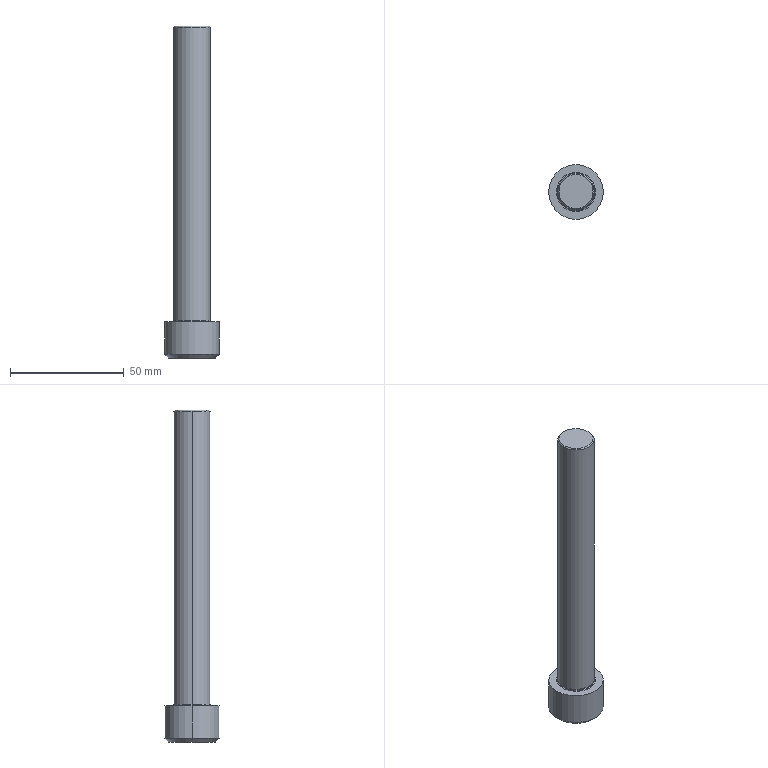Part | Creo | 1 solid | 23 faces | box 24 x 24 x 146 mm | volume 31613 mm3 | plane 9 | cone 6 | cylinder 4 | torus 4 | commonest cylinder face diameters 16 x2 24 x2
STEP:
#1=CARTESIAN_POINT('',(0.,0.,0.));
#2=DIRECTION('',(0.,0.,1.));
#3=DIRECTION('',(1.,0.,0.));
#4=AXIS2_PLACEMENT_3D('',#1,#2,#3);
#5=CARTESIAN_POINT('',(101.917,220.,10.5));
#6=VERTEX_POINT('',#5);
#7=CARTESIAN_POINT('',(105.959,227.,10.5));
#8=VERTEX_POINT('',#7);
#9=CARTESIAN_POINT('',(101.917,220.,10.5));
#10=CARTESIAN_POINT('',(102.137,220.381,10.627));
#11=CARTESIAN_POINT('',(102.578,221.145,10.851));
#12=CARTESIAN_POINT('',(103.254,222.315,11.073));
#13=CARTESIAN_POINT('',(103.936,223.496,11.151));
#14=CARTESIAN_POINT('',(104.621,224.683,11.073));
#15=CARTESIAN_POINT('',(105.295,225.85,10.852));
#16=CARTESIAN_POINT('',(105.738,226.618,10.627));
#17=CARTESIAN_POINT('',(105.959,227.,10.5));
#18=B_SPLINE_CURVE_WITH_KNOTS('',3,(#9,#10,#11,#12,#13,#14,#15,#16,#17),.UNSPECIFIED.,.F.,.F.,(4,1,1,1,1,1,4),(0.,0.1667,0.3333,0.5,0.6667,0.8333,1.),.UNSPECIFIED.);
#19=EDGE_CURVE('',#6,#8,#18,.T.);
#20=ORIENTED_EDGE('',*,*,#19,.F.);
#21=CARTESIAN_POINT('',(110.,220.,15.167));
#22=VERTEX_POINT('',#21);
#23=CARTESIAN_POINT('',(110.,220.,15.167));
#24=DIRECTION('',(-0.866,0.,-0.5));
#25=VECTOR('',#24,9.333);
#26=LINE('',#23,#25);
#27=EDGE_CURVE('',#22,#6,#26,.T.);
#28=ORIENTED_EDGE('',*,*,#27,.F.);
#29=CARTESIAN_POINT('',(118.083,220.,10.5));
#30=VERTEX_POINT('',#29);
#31=CARTESIAN_POINT('',(110.,220.,15.167));
#32=DIRECTION('',(0.866,0.,-0.5));
#33=VECTOR('',#32,9.333);
#34=LINE('',#31,#33);
#35=EDGE_CURVE('',#22,#30,#34,.T.);
#36=ORIENTED_EDGE('',*,*,#35,.T.);
#37=CARTESIAN_POINT('',(114.041,227.,10.5));
#38=VERTEX_POINT('',#37);
#39=CARTESIAN_POINT('',(114.041,227.,10.5));
#40=CARTESIAN_POINT('',(114.261,226.619,10.627));
#41=CARTESIAN_POINT('',(114.703,225.855,10.851));
#42=CARTESIAN_POINT('',(115.378,224.685,11.073));
#43=CARTESIAN_POINT('',(116.06,223.504,11.151));
#44=CARTESIAN_POINT('',(116.745,222.317,11.073));
#45=CARTESIAN_POINT('',(117.419,221.15,10.852));
#46=CARTESIAN_POINT('',(117.862,220.382,10.627));
#47=CARTESIAN_POINT('',(118.083,220.,10.5));
#48=B_SPLINE_CURVE_WITH_KNOTS('',3,(#39,#40,#41,#42,#43,#44,#45,#46,#47),.UNSPECIFIED.,.F.,.F.,(4,1,1,1,1,1,4),(0.,0.1667,0.3333,0.5,0.6667,0.8333,1.),.UNSPECIFIED.);
#49=EDGE_CURVE('',#38,#30,#48,.T.);
#50=ORIENTED_EDGE('',*,*,#49,.F.);
#51=CARTESIAN_POINT('',(105.959,227.,10.5));
#52=CARTESIAN_POINT('',(106.396,227.,10.626));
#53=CARTESIAN_POINT('',(107.277,227.,10.85));
#54=CARTESIAN_POINT('',(108.631,227.,11.073));
#55=CARTESIAN_POINT('',(109.998,227.,11.151));
#56=CARTESIAN_POINT('',(111.363,227.,11.074));
#57=CARTESIAN_POINT('',(112.717,227.,10.851));
#58=CARTESIAN_POINT('',(113.601,227.,10.627));
#59=CARTESIAN_POINT('',(114.041,227.,10.5));
#60=B_SPLINE_CURVE_WITH_KNOTS('',3,(#51,#52,#53,#54,#55,#56,#57,#58,#59),.UNSPECIFIED.,.F.,.F.,(4,1,1,1,1,1,4),(0.,0.1667,0.3333,0.5,0.6667,0.8333,1.),.UNSPECIFIED.);
#61=EDGE_CURVE('',#8,#38,#60,.T.);
#62=ORIENTED_EDGE('',*,*,#61,.F.);
#63=EDGE_LOOP('',(#20,#28,#36,#50,#62));
#64=FACE_OUTER_BOUND('',#63,.F.);
#65=CARTESIAN_POINT('',(110.,220.,12.787));
#66=DIRECTION('',(0.,0.,-1.));
#67=DIRECTION('',(-1.,0.,0.));
#68=AXIS2_PLACEMENT_3D('',#65,#66,#67);
#69=CONICAL_SURFACE('',#68,4.122,60.);
#70=ADVANCED_FACE('',(#64),#69,.F.);
#71=CARTESIAN_POINT('',(105.959,227.,2.5));
#72=VERTEX_POINT('',#71);
#73=CARTESIAN_POINT('',(101.917,220.,2.5));
#74=VERTEX_POINT('',#73);
#75=CARTESIAN_POINT('',(105.959,227.,2.5));
#76=DIRECTION('',(-0.5,-0.866,0.));
#77=VECTOR('',#76,8.083);
#78=LINE('',#75,#77);
#79=EDGE_CURVE('',#72,#74,#78,.T.);
#80=ORIENTED_EDGE('',*,*,#79,.T.);
#81=CARTESIAN_POINT('',(101.917,220.,2.5));
#82=DIRECTION('',(0.,0.,1.));
#83=VECTOR('',#82,8.);
#84=LINE('',#81,#83);
#85=EDGE_CURVE('',#74,#6,#84,.T.);
#86=ORIENTED_EDGE('',*,*,#85,.T.);
#87=ORIENTED_EDGE('',*,*,#19,.T.);
#88=CARTESIAN_POINT('',(105.959,227.,2.5));
#89=DIRECTION('',(0.,0.,1.));
#90=VECTOR('',#89,8.);
#91=LINE('',#88,#90);
#92=EDGE_CURVE('',#72,#8,#91,.T.);
#93=ORIENTED_EDGE('',*,*,#92,.F.);
#94=EDGE_LOOP('',(#80,#86,#87,#93));
#95=FACE_OUTER_BOUND('',#94,.F.);
#96=CARTESIAN_POINT('',(105.959,227.,10.5));
#97=DIRECTION('',(0.866,-0.5,0.));
#98=DIRECTION('',(-0.5,-0.866,0.));
#99=AXIS2_PLACEMENT_3D('',#96,#97,#98);
#100=PLANE('',#99);
#101=ADVANCED_FACE('',(#95),#100,.T.);
#102=CARTESIAN_POINT('',(99.6,220.,2.5));
#103=VERTEX_POINT('',#102);
#104=CARTESIAN_POINT('',(120.4,220.,2.5));
#105=VERTEX_POINT('',#104);
#106=CARTESIAN_POINT('',(110.,220.,2.5));
#107=DIRECTION('',(0.,0.,-1.));
#108=DIRECTION('',(-1.,0.,0.));
#109=AXIS2_PLACEMENT_3D('',#106,#107,#108);
#110=CIRCLE('',#109,10.4);
#111=EDGE_CURVE('',#103,#105,#110,.T.);
#112=ORIENTED_EDGE('',*,*,#111,.F.);
#113=CARTESIAN_POINT('',(110.,220.,2.5));
#114=DIRECTION('',(0.,0.,-1.));
#115=DIRECTION('',(1.,0.,0.));
#116=AXIS2_PLACEMENT_3D('',#113,#114,#115);
#117=CIRCLE('',#116,10.4);
#118=EDGE_CURVE('',#105,#103,#117,.T.);
#119=ORIENTED_EDGE('',*,*,#118,.F.);
#120=EDGE_LOOP('',(#112,#119));
#121=FACE_OUTER_BOUND('',#120,.F.);
#122=CARTESIAN_POINT('',(105.959,213.,2.5));
#123=VERTEX_POINT('',#122);
#124=CARTESIAN_POINT('',(101.917,220.,2.5));
#125=DIRECTION('',(0.5,-0.866,0.));
#126=VECTOR('',#125,8.083);
#127=LINE('',#124,#126);
#128=EDGE_CURVE('',#74,#123,#127,.T.);
#129=ORIENTED_EDGE('',*,*,#128,.F.);
#130=ORIENTED_EDGE('',*,*,#79,.F.);
#131=CARTESIAN_POINT('',(114.041,227.,2.5));
#132=VERTEX_POINT('',#131);
#133=CARTESIAN_POINT('',(105.959,227.,2.5));
#134=DIRECTION('',(1.,0.,0.));
#135=VECTOR('',#134,8.083);
#136=LINE('',#133,#135);
#137=EDGE_CURVE('',#72,#132,#136,.T.);
#138=ORIENTED_EDGE('',*,*,#137,.T.);
#139=CARTESIAN_POINT('',(118.083,220.,2.5));
#140=VERTEX_POINT('',#139);
#141=CARTESIAN_POINT('',(118.083,220.,2.5));
#142=DIRECTION('',(-0.5,0.866,0.));
#143=VECTOR('',#142,8.083);
#144=LINE('',#141,#143);
#145=EDGE_CURVE('',#140,#132,#144,.T.);
#146=ORIENTED_EDGE('',*,*,#145,.F.);
#147=CARTESIAN_POINT('',(114.041,213.,2.5));
#148=VERTEX_POINT('',#147);
#149=CARTESIAN_POINT('',(114.041,213.,2.5));
#150=DIRECTION('',(0.5,0.866,0.));
#151=VECTOR('',#150,8.083);
#152=LINE('',#149,#151);
#153=EDGE_CURVE('',#148,#140,#152,.T.);
#154=ORIENTED_EDGE('',*,*,#153,.F.);
#155=CARTESIAN_POINT('',(114.041,213.,2.5));
#156=DIRECTION('',(-1.,0.,0.));
#157=VECTOR('',#156,8.083);
#158=LINE('',#155,#157);
#159=EDGE_CURVE('',#148,#123,#158,.T.);
#160=ORIENTED_EDGE('',*,*,#159,.T.);
#161=EDGE_LOOP('',(#129,#130,#138,#146,#154,#160));
#162=FACE_BOUND('',#161,.F.);
#163=CARTESIAN_POINT('',(110.,220.,2.5));
#164=DIRECTION('',(0.,0.,-1.));
#165=DIRECTION('',(-1.,0.,0.));
#166=AXIS2_PLACEMENT_3D('',#163,#164,#165);
#167=PLANE('',#166);
#168=ADVANCED_FACE('',(#121,#162),#167,.T.);
#169=CARTESIAN_POINT('',(98.,220.,4.1));
#170=VERTEX_POINT('',#169);
#171=CARTESIAN_POINT('',(122.,220.,4.1));
#172=VERTEX_POINT('',#171);
#173=CARTESIAN_POINT('',(110.,220.,4.1));
#174=DIRECTION('',(0.,0.,-1.));
#175=DIRECTION('',(-1.,0.,0.));
#176=AXIS2_PLACEMENT_3D('',#173,#174,#175);
#177=CIRCLE('',#176,12.);
#178=EDGE_CURVE('',#170,#172,#177,.T.);
#179=ORIENTED_EDGE('',*,*,#178,.F.);
#180=CARTESIAN_POINT('',(99.6,220.,2.5));
#181=DIRECTION('',(-0.7071,0.,0.7071));
#182=VECTOR('',#181,2.263);
#183=LINE('',#180,#182);
#184=EDGE_CURVE('',#103,#170,#183,.T.);
#185=ORIENTED_EDGE('',*,*,#184,.F.);
#186=ORIENTED_EDGE('',*,*,#111,.T.);
#187=CARTESIAN_POINT('',(120.4,220.,2.5));
#188=DIRECTION('',(0.7071,0.,0.7071));
#189=VECTOR('',#188,2.263);
#190=LINE('',#187,#189);
#191=EDGE_CURVE('',#105,#172,#190,.T.);
#192=ORIENTED_EDGE('',*,*,#191,.T.);
#193=EDGE_LOOP('',(#179,#185,#186,#192));
#194=FACE_OUTER_BOUND('',#193,.F.);
#195=CARTESIAN_POINT('',(110.,220.,3.3));
#196=DIRECTION('',(0.,0.,1.));
#197=DIRECTION('',(1.,0.,0.));
#198=AXIS2_PLACEMENT_3D('',#195,#196,#197);
#199=CONICAL_SURFACE('',#198,11.2,45.);
#200=ADVANCED_FACE('',(#194),#199,.T.);
#201=ORIENTED_EDGE('',*,*,#178,.T.);
#202=CARTESIAN_POINT('',(122.,220.,18.5));
#203=VERTEX_POINT('',#202);
#204=CARTESIAN_POINT('',(122.,220.,18.5));
#205=DIRECTION('',(0.,0.,-1.));
#206=VECTOR('',#205,14.4);
#207=LINE('',#204,#206);
#208=EDGE_CURVE('',#203,#172,#207,.T.);
#209=ORIENTED_EDGE('',*,*,#208,.F.);
#210=CARTESIAN_POINT('',(98.,220.,18.5));
#211=VERTEX_POINT('',#210);
#212=CARTESIAN_POINT('',(110.,220.,18.5));
#213=DIRECTION('',(0.,0.,1.));
#214=DIRECTION('',(1.,0.,0.));
#215=AXIS2_PLACEMENT_3D('',#212,#213,#214);
#216=CIRCLE('',#215,12.);
#217=EDGE_CURVE('',#203,#211,#216,.T.);
#218=ORIENTED_EDGE('',*,*,#217,.T.);
#219=CARTESIAN_POINT('',(98.,220.,18.5));
#220=DIRECTION('',(0.,0.,-1.));
#221=VECTOR('',#220,14.4);
#222=LINE('',#219,#221);
#223=EDGE_CURVE('',#211,#170,#222,.T.);
#224=ORIENTED_EDGE('',*,*,#223,.T.);
#225=EDGE_LOOP('',(#201,#209,#218,#224));
#226=FACE_OUTER_BOUND('',#225,.F.);
#227=CARTESIAN_POINT('',(110.,220.,18.5));
#228=DIRECTION('',(0.,0.,-1.));
#229=DIRECTION('',(-1.,0.,0.));
#230=AXIS2_PLACEMENT_3D('',#227,#228,#229);
#231=CYLINDRICAL_SURFACE('',#230,12.);
#232=ADVANCED_FACE('',(#226),#231,.T.);
#233=CARTESIAN_POINT('',(110.,220.,4.1));
#234=DIRECTION('',(0.,0.,-1.));
#235=DIRECTION('',(1.,0.,0.));
#236=AXIS2_PLACEMENT_3D('',#233,#234,#235);
#237=CIRCLE('',#236,12.);
#238=EDGE_CURVE('',#172,#170,#237,.T.);
#239=ORIENTED_EDGE('',*,*,#238,.T.);
#240=ORIENTED_EDGE('',*,*,#223,.F.);
#241=CARTESIAN_POINT('',(110.,220.,18.5));
#242=DIRECTION('',(0.,0.,1.));
#243=DIRECTION('',(-1.,0.,0.));
#244=AXIS2_PLACEMENT_3D('',#241,#242,#243);
#245=CIRCLE('',#244,12.);
#246=EDGE_CURVE('',#211,#203,#245,.T.);
#247=ORIENTED_EDGE('',*,*,#246,.T.);
#248=ORIENTED_EDGE('',*,*,#208,.T.);
#249=EDGE_LOOP('',(#239,#240,#247,#248));
#250=FACE_OUTER_BOUND('',#249,.F.);
#251=CARTESIAN_POINT('',(110.,220.,18.5));
#252=DIRECTION('',(0.,0.,-1.));
#253=DIRECTION('',(-1.,0.,0.));
#254=AXIS2_PLACEMENT_3D('',#251,#252,#253);
#255=CYLINDRICAL_SURFACE('',#254,12.);
#256=ADVANCED_FACE('',(#250),#255,.T.);
#257=ORIENTED_EDGE('',*,*,#238,.F.);
#258=ORIENTED_EDGE('',*,*,#191,.F.);
#259=ORIENTED_EDGE('',*,*,#118,.T.);
#260=ORIENTED_EDGE('',*,*,#184,.T.);
#261=EDGE_LOOP('',(#257,#258,#259,#260));
#262=FACE_OUTER_BOUND('',#261,.F.);
#263=CARTESIAN_POINT('',(110.,220.,3.3));
#264=DIRECTION('',(0.,0.,1.));
#265=DIRECTION('',(1.,0.,0.));
#266=AXIS2_PLACEMENT_3D('',#263,#264,#265);
#267=CONICAL_SURFACE('',#266,11.2,45.);
#268=ADVANCED_FACE('',(#262),#267,.T.);
#269=ORIENTED_EDGE('',*,*,#246,.F.);
#270=ORIENTED_EDGE('',*,*,#217,.F.);
#271=EDGE_LOOP('',(#269,#270));
#272=FACE_OUTER_BOUND('',#271,.F.);
#273=CARTESIAN_POINT('',(101.4,220.,18.5));
#274=VERTEX_POINT('',#273);
#275=CARTESIAN_POINT('',(118.6,220.,18.5));
#276=VERTEX_POINT('',#275);
#277=CARTESIAN_POINT('',(110.,220.,18.5));
#278=DIRECTION('',(0.,0.,-1.));
#279=DIRECTION('',(-1.,0.,0.));
#280=AXIS2_PLACEMENT_3D('',#277,#278,#279);
#281=CIRCLE('',#280,8.6);
#282=EDGE_CURVE('',#274,#276,#281,.T.);
#283=ORIENTED_EDGE('',*,*,#282,.F.);
#284=CARTESIAN_POINT('',(110.,220.,18.5));
#285=DIRECTION('',(0.,0.,-1.));
#286=DIRECTION('',(1.,0.,0.));
#287=AXIS2_PLACEMENT_3D('',#284,#285,#286);
#288=CIRCLE('',#287,8.6);
#289=EDGE_CURVE('',#276,#274,#288,.T.);
#290=ORIENTED_EDGE('',*,*,#289,.F.);
#291=EDGE_LOOP('',(#283,#290));
#292=FACE_BOUND('',#291,.F.);
#293=CARTESIAN_POINT('',(110.,220.,18.5));
#294=DIRECTION('',(0.,0.,-1.));
#295=DIRECTION('',(-1.,0.,0.));
#296=AXIS2_PLACEMENT_3D('',#293,#294,#295);
#297=PLANE('',#296);
#298=ADVANCED_FACE('',(#272,#292),#297,.F.);
#299=ORIENTED_EDGE('',*,*,#282,.T.);
#300=CARTESIAN_POINT('',(118.176,220.,18.676));
#301=VERTEX_POINT('',#300);
#302=CARTESIAN_POINT('',(118.6,220.,19.1));
#303=DIRECTION('',(0.,1.,0.));
#304=DIRECTION('',(0.,0.,-1.));
#305=AXIS2_PLACEMENT_3D('',#302,#303,#304);
#306=CIRCLE('',#305,0.6);
#307=EDGE_CURVE('',#276,#301,#306,.T.);
#308=ORIENTED_EDGE('',*,*,#307,.T.);
#309=CARTESIAN_POINT('',(101.824,220.,18.676));
#310=VERTEX_POINT('',#309);
#311=CARTESIAN_POINT('',(110.,220.,18.676));
#312=DIRECTION('',(0.,0.,-1.));
#313=DIRECTION('',(-1.,0.,0.));
#314=AXIS2_PLACEMENT_3D('',#311,#312,#313);
#315=CIRCLE('',#314,8.176);
#316=EDGE_CURVE('',#310,#301,#315,.T.);
#317=ORIENTED_EDGE('',*,*,#316,.F.);
#318=CARTESIAN_POINT('',(101.4,220.,19.1));
#319=DIRECTION('',(0.,-1.,0.));
#320=DIRECTION('',(0.,0.,-1.));
#321=AXIS2_PLACEMENT_3D('',#318,#319,#320);
#322=CIRCLE('',#321,0.6);
#323=EDGE_CURVE('',#274,#310,#322,.T.);
#324=ORIENTED_EDGE('',*,*,#323,.F.);
#325=EDGE_LOOP('',(#299,#308,#317,#324));
#326=FACE_OUTER_BOUND('',#325,.F.);
#327=CARTESIAN_POINT('',(110.,220.,19.1));
#328=DIRECTION('',(0.,0.,-1.));
#329=DIRECTION('',(-1.,0.,0.));
#330=AXIS2_PLACEMENT_3D('',#327,#328,#329);
#331=TOROIDAL_SURFACE('',#330,8.6,0.6);
#332=ADVANCED_FACE('',(#326),#331,.F.);
#333=ORIENTED_EDGE('',*,*,#289,.T.);
#334=ORIENTED_EDGE('',*,*,#323,.T.);
#335=CARTESIAN_POINT('',(110.,220.,18.676));
#336=DIRECTION('',(0.,0.,-1.));
#337=DIRECTION('',(1.,0.,0.));
#338=AXIS2_PLACEMENT_3D('',#335,#336,#337);
#339=CIRCLE('',#338,8.176);
#340=EDGE_CURVE('',#301,#310,#339,.T.);
#341=ORIENTED_EDGE('',*,*,#340,.F.);
#342=ORIENTED_EDGE('',*,*,#307,.F.);
#343=EDGE_LOOP('',(#333,#334,#341,#342));
#344=FACE_OUTER_BOUND('',#343,.F.);
#345=CARTESIAN_POINT('',(110.,220.,19.1));
#346=DIRECTION('',(0.,0.,-1.));
#347=DIRECTION('',(-1.,0.,0.));
#348=AXIS2_PLACEMENT_3D('',#345,#346,#347);
#349=TOROIDAL_SURFACE('',#348,8.6,0.6);
#350=ADVANCED_FACE('',(#344),#349,.F.);
#351=CARTESIAN_POINT('',(118.,220.,19.1));
#352=VERTEX_POINT('',#351);
#353=CARTESIAN_POINT('',(102.,220.,19.1));
#354=VERTEX_POINT('',#353);
#355=CARTESIAN_POINT('',(110.,220.,19.1));
#356=DIRECTION('',(0.,0.,-1.));
#357=DIRECTION('',(1.,0.,0.));
#358=AXIS2_PLACEMENT_3D('',#355,#356,#357);
#359=CIRCLE('',#358,8.);
#360=EDGE_CURVE('',#352,#354,#359,.T.);
#361=ORIENTED_EDGE('',*,*,#360,.F.);
#362=CARTESIAN_POINT('',(118.6,220.,19.1));
#363=DIRECTION('',(0.,1.,0.));
#364=DIRECTION('',(-0.7071,0.,-0.7071));
#365=AXIS2_PLACEMENT_3D('',#362,#363,#364);
#366=CIRCLE('',#365,0.6);
#367=EDGE_CURVE('',#301,#352,#366,.T.);
#368=ORIENTED_EDGE('',*,*,#367,.F.);
#369=ORIENTED_EDGE('',*,*,#340,.T.);
#370=CARTESIAN_POINT('',(101.4,220.,19.1));
#371=DIRECTION('',(0.,-1.,0.));
#372=DIRECTION('',(0.7071,0.,-0.7071));
#373=AXIS2_PLACEMENT_3D('',#370,#371,#372);
#374=CIRCLE('',#373,0.6);
#375=EDGE_CURVE('',#310,#354,#374,.T.);
#376=ORIENTED_EDGE('',*,*,#375,.T.);
#377=EDGE_LOOP('',(#361,#368,#369,#376));
#378=FACE_OUTER_BOUND('',#377,.F.);
#379=CARTESIAN_POINT('',(110.,220.,19.1));
#380=DIRECTION('',(0.,0.,-1.));
#381=DIRECTION('',(-1.,0.,0.));
#382=AXIS2_PLACEMENT_3D('',#379,#380,#381);
#383=TOROIDAL_SURFACE('',#382,8.6,0.6);
#384=ADVANCED_FACE('',(#378),#383,.F.);
#385=CARTESIAN_POINT('',(102.,220.,148.));
#386=VERTEX_POINT('',#385);
#387=CARTESIAN_POINT('',(118.,220.,148.));
#388=VERTEX_POINT('',#387);
#389=CARTESIAN_POINT('',(110.,220.,148.));
#390=DIRECTION('',(0.,0.,1.));
#391=DIRECTION('',(-1.,0.,0.));
#392=AXIS2_PLACEMENT_3D('',#389,#390,#391);
#393=CIRCLE('',#392,8.);
#394=EDGE_CURVE('',#386,#388,#393,.T.);
#395=ORIENTED_EDGE('',*,*,#394,.T.);
#396=CARTESIAN_POINT('',(118.,220.,148.));
#397=DIRECTION('',(0.,0.,-1.));
#398=VECTOR('',#397,128.9);
#399=LINE('',#396,#398);
#400=EDGE_CURVE('',#388,#352,#399,.T.);
#401=ORIENTED_EDGE('',*,*,#400,.T.);
#402=ORIENTED_EDGE('',*,*,#360,.T.);
#403=CARTESIAN_POINT('',(102.,220.,148.));
#404=DIRECTION('',(0.,0.,-1.));
#405=VECTOR('',#404,128.9);
#406=LINE('',#403,#405);
#407=EDGE_CURVE('',#386,#354,#406,.T.);
#408=ORIENTED_EDGE('',*,*,#407,.F.);
#409=EDGE_LOOP('',(#395,#401,#402,#408));
#410=FACE_OUTER_BOUND('',#409,.F.);
#411=CARTESIAN_POINT('',(110.,220.,148.5));
#412=DIRECTION('',(0.,0.,-1.));
#413=DIRECTION('',(-1.,0.,0.));
#414=AXIS2_PLACEMENT_3D('',#411,#412,#413);
#415=CYLINDRICAL_SURFACE('',#414,8.);
#416=ADVANCED_FACE('',(#410),#415,.T.);
#417=CARTESIAN_POINT('',(102.5,220.,148.5));
#418=VERTEX_POINT('',#417);
#419=CARTESIAN_POINT('',(117.5,220.,148.5));
#420=VERTEX_POINT('',#419);
#421=CARTESIAN_POINT('',(110.,220.,148.5));
#422=DIRECTION('',(0.,0.,1.));
#423=DIRECTION('',(-1.,0.,0.));
#424=AXIS2_PLACEMENT_3D('',#421,#422,#423);
#425=CIRCLE('',#424,7.5);
#426=EDGE_CURVE('',#418,#420,#425,.T.);
#427=ORIENTED_EDGE('',*,*,#426,.T.);
#428=CARTESIAN_POINT('',(117.5,220.,148.5));
#429=DIRECTION('',(0.7071,0.,-0.7071));
#430=VECTOR('',#429,0.7071);
#431=LINE('',#428,#430);
#432=EDGE_CURVE('',#420,#388,#431,.T.);
#433=ORIENTED_EDGE('',*,*,#432,.T.);
#434=ORIENTED_EDGE('',*,*,#394,.F.);
#435=CARTESIAN_POINT('',(102.5,220.,148.5));
#436=DIRECTION('',(-0.7071,0.,-0.7071));
#437=VECTOR('',#436,0.7071);
#438=LINE('',#435,#437);
#439=EDGE_CURVE('',#418,#386,#438,.T.);
#440=ORIENTED_EDGE('',*,*,#439,.F.);
#441=EDGE_LOOP('',(#427,#433,#434,#440));
#442=FACE_OUTER_BOUND('',#441,.F.);
#443=CARTESIAN_POINT('',(110.,220.,148.25));
#444=DIRECTION('',(0.,0.,-1.));
#445=DIRECTION('',(-1.,0.,0.));
#446=AXIS2_PLACEMENT_3D('',#443,#444,#445);
#447=CONICAL_SURFACE('',#446,7.75,45.);
#448=ADVANCED_FACE('',(#442),#447,.T.);
#449=ORIENTED_EDGE('',*,*,#426,.F.);
#450=CARTESIAN_POINT('',(110.,220.,148.5));
#451=DIRECTION('',(0.,0.,1.));
#452=DIRECTION('',(1.,0.,0.));
#453=AXIS2_PLACEMENT_3D('',#450,#451,#452);
#454=CIRCLE('',#453,7.5);
#455=EDGE_CURVE('',#420,#418,#454,.T.);
#456=ORIENTED_EDGE('',*,*,#455,.F.);
#457=EDGE_LOOP('',(#449,#456));
#458=FACE_OUTER_BOUND('',#457,.F.);
#459=CARTESIAN_POINT('',(110.,220.,148.5));
#460=DIRECTION('',(0.,0.,-1.));
#461=DIRECTION('',(-1.,0.,0.));
#462=AXIS2_PLACEMENT_3D('',#459,#460,#461);
#463=PLANE('',#462);
#464=ADVANCED_FACE('',(#458),#463,.F.);
#465=ORIENTED_EDGE('',*,*,#455,.T.);
#466=ORIENTED_EDGE('',*,*,#439,.T.);
#467=CARTESIAN_POINT('',(110.,220.,148.));
#468=DIRECTION('',(0.,0.,1.));
#469=DIRECTION('',(1.,0.,0.));
#470=AXIS2_PLACEMENT_3D('',#467,#468,#469);
#471=CIRCLE('',#470,8.);
#472=EDGE_CURVE('',#388,#386,#471,.T.);
#473=ORIENTED_EDGE('',*,*,#472,.F.);
#474=ORIENTED_EDGE('',*,*,#432,.F.);
#475=EDGE_LOOP('',(#465,#466,#473,#474));
#476=FACE_OUTER_BOUND('',#475,.F.);
#477=CARTESIAN_POINT('',(110.,220.,148.25));
#478=DIRECTION('',(0.,0.,-1.));
#479=DIRECTION('',(-1.,0.,0.));
#480=AXIS2_PLACEMENT_3D('',#477,#478,#479);
#481=CONICAL_SURFACE('',#480,7.75,45.);
#482=ADVANCED_FACE('',(#476),#481,.T.);
#483=ORIENTED_EDGE('',*,*,#472,.T.);
#484=ORIENTED_EDGE('',*,*,#407,.T.);
#485=CARTESIAN_POINT('',(110.,220.,19.1));
#486=DIRECTION('',(0.,0.,-1.));
#487=DIRECTION('',(-1.,0.,0.));
#488=AXIS2_PLACEMENT_3D('',#485,#486,#487);
#489=CIRCLE('',#488,8.);
#490=EDGE_CURVE('',#354,#352,#489,.T.);
#491=ORIENTED_EDGE('',*,*,#490,.T.);
#492=ORIENTED_EDGE('',*,*,#400,.F.);
#493=EDGE_LOOP('',(#483,#484,#491,#492));
#494=FACE_OUTER_BOUND('',#493,.F.);
#495=CARTESIAN_POINT('',(110.,220.,148.5));
#496=DIRECTION('',(0.,0.,-1.));
#497=DIRECTION('',(-1.,0.,0.));
#498=AXIS2_PLACEMENT_3D('',#495,#496,#497);
#499=CYLINDRICAL_SURFACE('',#498,8.);
#500=ADVANCED_FACE('',(#494),#499,.T.);
#501=ORIENTED_EDGE('',*,*,#490,.F.);
#502=ORIENTED_EDGE('',*,*,#375,.F.);
#503=ORIENTED_EDGE('',*,*,#316,.T.);
#504=ORIENTED_EDGE('',*,*,#367,.T.);
#505=EDGE_LOOP('',(#501,#502,#503,#504));
#506=FACE_OUTER_BOUND('',#505,.F.);
#507=CARTESIAN_POINT('',(110.,220.,19.1));
#508=DIRECTION('',(0.,0.,-1.));
#509=DIRECTION('',(-1.,0.,0.));
#510=AXIS2_PLACEMENT_3D('',#507,#508,#509);
#511=TOROIDAL_SURFACE('',#510,8.6,0.6);
#512=ADVANCED_FACE('',(#506),#511,.F.);
#513=ORIENTED_EDGE('',*,*,#128,.T.);
#514=CARTESIAN_POINT('',(105.959,213.,10.5));
#515=VERTEX_POINT('',#514);
#516=CARTESIAN_POINT('',(105.959,213.,2.5));
#517=DIRECTION('',(0.,0.,1.));
#518=VECTOR('',#517,8.);
#519=LINE('',#516,#518);
#520=EDGE_CURVE('',#123,#515,#519,.T.);
#521=ORIENTED_EDGE('',*,*,#520,.T.);
#522=CARTESIAN_POINT('',(105.959,213.,10.5));
#523=CARTESIAN_POINT('',(105.739,213.381,10.627));
#524=CARTESIAN_POINT('',(105.297,214.145,10.851));
#525=CARTESIAN_POINT('',(104.622,215.315,11.073));
#526=CARTESIAN_POINT('',(103.94,216.496,11.151));
#527=CARTESIAN_POINT('',(103.255,217.683,11.073));
#528=CARTESIAN_POINT('',(102.581,218.85,10.852));
#529=CARTESIAN_POINT('',(102.138,219.618,10.627));
#530=CARTESIAN_POINT('',(101.917,220.,10.5));
#531=B_SPLINE_CURVE_WITH_KNOTS('',3,(#522,#523,#524,#525,#526,#527,#528,#529,#530),.UNSPECIFIED.,.F.,.F.,(4,1,1,1,1,1,4),(0.,0.1667,0.3333,0.5,0.6667,0.8333,1.),.UNSPECIFIED.);
#532=EDGE_CURVE('',#515,#6,#531,.T.);
#533=ORIENTED_EDGE('',*,*,#532,.T.);
#534=ORIENTED_EDGE('',*,*,#85,.F.);
#535=EDGE_LOOP('',(#513,#521,#533,#534));
#536=FACE_OUTER_BOUND('',#535,.F.);
#537=CARTESIAN_POINT('',(101.917,220.,10.5));
#538=DIRECTION('',(0.866,0.5,0.));
#539=DIRECTION('',(0.5,-0.866,0.));
#540=AXIS2_PLACEMENT_3D('',#537,#538,#539);
#541=PLANE('',#540);
#542=ADVANCED_FACE('',(#536),#541,.T.);
#543=ORIENTED_EDGE('',*,*,#159,.F.);
#544=CARTESIAN_POINT('',(114.041,213.,10.5));
#545=VERTEX_POINT('',#544);
#546=CARTESIAN_POINT('',(114.041,213.,2.5));
#547=DIRECTION('',(0.,0.,1.));
#548=VECTOR('',#547,8.);
#549=LINE('',#546,#548);
#550=EDGE_CURVE('',#148,#545,#549,.T.);
#551=ORIENTED_EDGE('',*,*,#550,.T.);
#552=CARTESIAN_POINT('',(114.041,213.,10.5));
#553=CARTESIAN_POINT('',(113.601,213.,10.627));
#554=CARTESIAN_POINT('',(112.717,213.,10.851));
#555=CARTESIAN_POINT('',(111.363,213.,11.074));
#556=CARTESIAN_POINT('',(109.998,213.,11.151));
#557=CARTESIAN_POINT('',(108.631,213.,11.073));
#558=CARTESIAN_POINT('',(107.277,213.,10.85));
#559=CARTESIAN_POINT('',(106.396,213.,10.626));
#560=CARTESIAN_POINT('',(105.959,213.,10.5));
#561=B_SPLINE_CURVE_WITH_KNOTS('',3,(#552,#553,#554,#555,#556,#557,#558,#559,#560),.UNSPECIFIED.,.F.,.F.,(4,1,1,1,1,1,4),(0.,0.1667,0.3333,0.5,0.6667,0.8333,1.),.UNSPECIFIED.);
#562=EDGE_CURVE('',#545,#515,#561,.T.);
#563=ORIENTED_EDGE('',*,*,#562,.T.);
#564=ORIENTED_EDGE('',*,*,#520,.F.);
#565=EDGE_LOOP('',(#543,#551,#563,#564));
#566=FACE_OUTER_BOUND('',#565,.F.);
#567=CARTESIAN_POINT('',(105.959,213.,10.5));
#568=DIRECTION('',(0.,1.,0.));
#569=DIRECTION('',(0.,0.,-1.));
#570=AXIS2_PLACEMENT_3D('',#567,#568,#569);
#571=PLANE('',#570);
#572=ADVANCED_FACE('',(#566),#571,.T.);
#573=ORIENTED_EDGE('',*,*,#153,.T.);
#574=CARTESIAN_POINT('',(118.083,220.,2.5));
#575=DIRECTION('',(0.,0.,1.));
#576=VECTOR('',#575,8.);
#577=LINE('',#574,#576);
#578=EDGE_CURVE('',#140,#30,#577,.T.);
#579=ORIENTED_EDGE('',*,*,#578,.T.);
#580=CARTESIAN_POINT('',(118.083,220.,10.5));
#581=CARTESIAN_POINT('',(117.862,219.618,10.627));
#582=CARTESIAN_POINT('',(117.419,218.85,10.852));
#583=CARTESIAN_POINT('',(116.745,217.683,11.073));
#584=CARTESIAN_POINT('',(116.06,216.496,11.151));
#585=CARTESIAN_POINT('',(115.378,215.315,11.073));
#586=CARTESIAN_POINT('',(114.703,214.145,10.851));
#587=CARTESIAN_POINT('',(114.261,213.381,10.627));
#588=CARTESIAN_POINT('',(114.041,213.,10.5));
#589=B_SPLINE_CURVE_WITH_KNOTS('',3,(#580,#581,#582,#583,#584,#585,#586,#587,#588),.UNSPECIFIED.,.F.,.F.,(4,1,1,1,1,1,4),(0.,0.1667,0.3333,0.5,0.6667,0.8333,1.),.UNSPECIFIED.);
#590=EDGE_CURVE('',#30,#545,#589,.T.);
#591=ORIENTED_EDGE('',*,*,#590,.T.);
#592=ORIENTED_EDGE('',*,*,#550,.F.);
#593=EDGE_LOOP('',(#573,#579,#591,#592));
#594=FACE_OUTER_BOUND('',#593,.F.);
#595=CARTESIAN_POINT('',(114.041,213.,10.5));
#596=DIRECTION('',(-0.866,0.5,0.));
#597=DIRECTION('',(0.5,0.866,0.));
#598=AXIS2_PLACEMENT_3D('',#595,#596,#597);
#599=PLANE('',#598);
#600=ADVANCED_FACE('',(#594),#599,.T.);
#601=ORIENTED_EDGE('',*,*,#145,.T.);
#602=CARTESIAN_POINT('',(114.041,227.,2.5));
#603=DIRECTION('',(0.,0.,1.));
#604=VECTOR('',#603,8.);
#605=LINE('',#602,#604);
#606=EDGE_CURVE('',#132,#38,#605,.T.);
#607=ORIENTED_EDGE('',*,*,#606,.T.);
#608=ORIENTED_EDGE('',*,*,#49,.T.);
#609=ORIENTED_EDGE('',*,*,#578,.F.);
#610=EDGE_LOOP('',(#601,#607,#608,#609));
#611=FACE_OUTER_BOUND('',#610,.F.);
#612=CARTESIAN_POINT('',(118.083,220.,10.5));
#613=DIRECTION('',(-0.866,-0.5,0.));
#614=DIRECTION('',(-0.5,0.866,0.));
#615=AXIS2_PLACEMENT_3D('',#612,#613,#614);
#616=PLANE('',#615);
#617=ADVANCED_FACE('',(#611),#616,.T.);
#618=ORIENTED_EDGE('',*,*,#137,.F.);
#619=ORIENTED_EDGE('',*,*,#92,.T.);
#620=ORIENTED_EDGE('',*,*,#61,.T.);
#621=ORIENTED_EDGE('',*,*,#606,.F.);
#622=EDGE_LOOP('',(#618,#619,#620,#621));
#623=FACE_OUTER_BOUND('',#622,.F.);
#624=CARTESIAN_POINT('',(114.041,227.,10.5));
#625=DIRECTION('',(0.,-1.,0.));
#626=DIRECTION('',(0.,0.,1.));
#627=AXIS2_PLACEMENT_3D('',#624,#625,#626);
#628=PLANE('',#627);
#629=ADVANCED_FACE('',(#623),#628,.T.);
#630=ORIENTED_EDGE('',*,*,#590,.F.);
#631=ORIENTED_EDGE('',*,*,#35,.F.);
#632=ORIENTED_EDGE('',*,*,#27,.T.);
#633=ORIENTED_EDGE('',*,*,#532,.F.);
#634=ORIENTED_EDGE('',*,*,#562,.F.);
#635=EDGE_LOOP('',(#630,#631,#632,#633,#634));
#636=FACE_OUTER_BOUND('',#635,.F.);
#637=CARTESIAN_POINT('',(110.,220.,12.787));
#638=DIRECTION('',(0.,0.,-1.));
#639=DIRECTION('',(-1.,0.,0.));
#640=AXIS2_PLACEMENT_3D('',#637,#638,#639);
#641=CONICAL_SURFACE('',#640,4.122,60.);
#642=ADVANCED_FACE('',(#636),#641,.F.);
#643=CLOSED_SHELL('',(#70,#101,#168,#200,#232,#256,#268,#298,#332,#350,#384,#416,#448,#464,#482,#500,#512,#542,#572,#600,#617,#629,#642));
#644=MANIFOLD_SOLID_BREP('',#643);
#645=(LENGTH_UNIT()NAMED_UNIT(*)SI_UNIT(.MILLI.,.METRE.));
#646=UNCERTAINTY_MEASURE_WITH_UNIT(LENGTH_MEASURE(0.01499),#645,'','');
#647=(NAMED_UNIT(*)PLANE_ANGLE_UNIT()SI_UNIT($,.RADIAN.));
#648=PLANE_ANGLE_MEASURE_WITH_UNIT(PLANE_ANGLE_MEASURE(0.01745),#647);
#649=(CONVERSION_BASED_UNIT('DEGREE',#648)NAMED_UNIT(*)PLANE_ANGLE_UNIT());
#650=(NAMED_UNIT(*)SI_UNIT($,.STERADIAN.)SOLID_ANGLE_UNIT());
#651=(GEOMETRIC_REPRESENTATION_CONTEXT(3)GLOBAL_UNCERTAINTY_ASSIGNED_CONTEXT((#646))GLOBAL_UNIT_ASSIGNED_CONTEXT((#645,#649,#650))REPRESENTATION_CONTEXT('',''));
#652=ADVANCED_BREP_SHAPE_REPRESENTATION('',(#4,#644),#651);